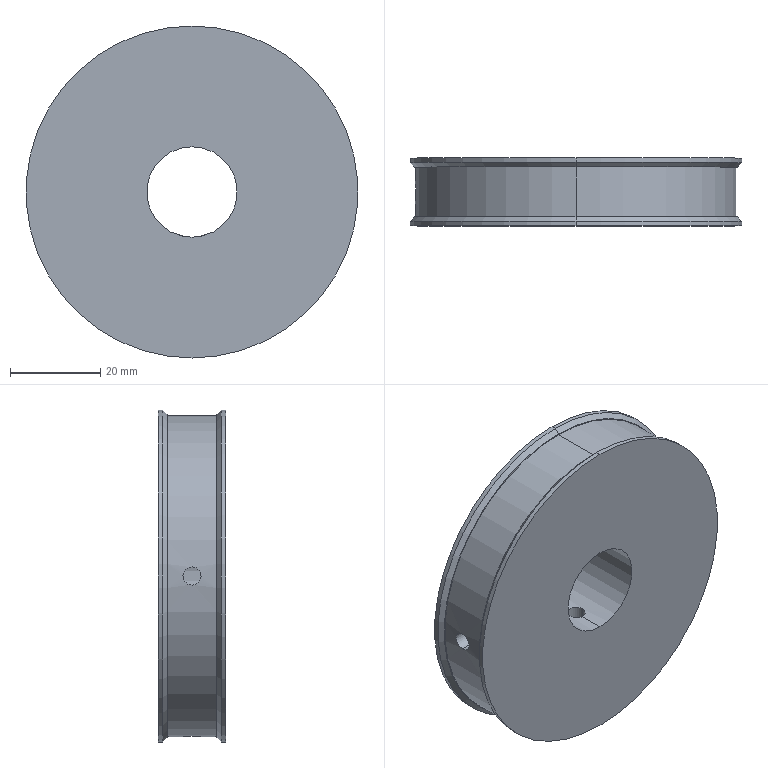Part | SolidWorks | features ICE 4, Chamfer 1, Extrusion 1 | 1 solid | 20 faces | box 73.4 x 15 x 73.4 mm | volume 54894 mm3 | cylinder 12 | cone 4 | plane 4 | commonest cylinder face diameters 4 x4 73.4 x4 20 x2 71 x2
STEP:
#1=CARTESIAN_POINT('',(-35.444,5.5,2.));
#2=VERTEX_POINT('',#1);
#3=CARTESIAN_POINT('',(-35.444,5.5,-2.));
#4=VERTEX_POINT('',#3);
#5=CARTESIAN_POINT('',(-35.444,5.5,2.));
#6=CARTESIAN_POINT('',(-35.444,5.239,2.));
#7=CARTESIAN_POINT('',(-35.447,4.976,1.948));
#8=CARTESIAN_POINT('',(-35.457,4.494,1.748));
#9=CARTESIAN_POINT('',(-35.464,4.271,1.599));
#10=CARTESIAN_POINT('',(-35.475,3.995,1.323));
#11=CARTESIAN_POINT('',(-35.479,3.91,1.22));
#12=CARTESIAN_POINT('',(-35.486,3.765,1.003));
#13=CARTESIAN_POINT('',(-35.489,3.703,0.8881));
#14=CARTESIAN_POINT('',(-35.494,3.603,0.6462));
#15=CARTESIAN_POINT('',(-35.496,3.564,0.5191));
#16=CARTESIAN_POINT('',(-35.499,3.513,0.2634));
#17=CARTESIAN_POINT('',(-35.5,3.5,0.1336));
#18=CARTESIAN_POINT('',(-35.5,3.5,-0.1303));
#19=CARTESIAN_POINT('',(-35.499,3.513,-0.2607));
#20=CARTESIAN_POINT('',(-35.496,3.563,-0.5163));
#21=CARTESIAN_POINT('',(-35.494,3.602,-0.6431));
#22=CARTESIAN_POINT('',(-35.489,3.702,-0.8856));
#23=CARTESIAN_POINT('',(-35.486,3.763,-1.001));
#24=CARTESIAN_POINT('',(-35.479,3.908,-1.218));
#25=CARTESIAN_POINT('',(-35.476,3.993,-1.321));
#26=CARTESIAN_POINT('',(-35.468,4.177,-1.506));
#27=CARTESIAN_POINT('',(-35.465,4.278,-1.588));
#28=CARTESIAN_POINT('',(-35.458,4.496,-1.735));
#29=CARTESIAN_POINT('',(-35.455,4.612,-1.797));
#30=CARTESIAN_POINT('',(-35.447,4.973,-1.947));
#31=CARTESIAN_POINT('',(-35.444,5.236,-2.));
#32=CARTESIAN_POINT('',(-35.444,5.5,-2.));
#33=B_SPLINE_CURVE_WITH_KNOTS('',3,(#5,#6,#7,#8,#9,#10,#11,#12,#13,#14,#15,#16,#17,#18,#19,#20,#21,#22,#23,#24,#25,#26,#27,#28,#29,#30,#31,#32),.UNSPECIFIED.,.F.,.F.,(4,2,2,2,2,2,2,2,2,2,2,2,2,4),(0.006254,0.007036,0.007817,0.008208,0.008599,0.00899,0.009381,0.009771,0.01016,0.01055,0.01094,0.01133,0.01173,0.01251),.UNSPECIFIED.);
#34=EDGE_CURVE('',#2,#4,#33,.T.);
#35=ORIENTED_EDGE('',*,*,#34,.F.);
#36=CARTESIAN_POINT('',(-9.798,5.5,2.));
#37=VERTEX_POINT('',#36);
#38=CARTESIAN_POINT('',(-43.,5.5,2.));
#39=DIRECTION('',(1.,0.,0.));
#40=VECTOR('',#39,1000.);
#41=LINE('',#38,#40);
#42=EDGE_CURVE('',#2,#37,#41,.T.);
#43=ORIENTED_EDGE('',*,*,#42,.T.);
#44=CARTESIAN_POINT('',(-9.798,5.5,-2.));
#45=VERTEX_POINT('',#44);
#46=CARTESIAN_POINT('',(-9.798,5.5,2.));
#47=CARTESIAN_POINT('',(-9.798,5.239,2.));
#48=CARTESIAN_POINT('',(-9.809,4.975,1.947));
#49=CARTESIAN_POINT('',(-9.837,4.614,1.798));
#50=CARTESIAN_POINT('',(-9.849,4.497,1.735));
#51=CARTESIAN_POINT('',(-9.873,4.279,1.59));
#52=CARTESIAN_POINT('',(-9.886,4.179,1.507));
#53=CARTESIAN_POINT('',(-9.913,3.994,1.323));
#54=CARTESIAN_POINT('',(-9.926,3.91,1.22));
#55=CARTESIAN_POINT('',(-9.95,3.765,1.004));
#56=CARTESIAN_POINT('',(-9.961,3.704,0.8892));
#57=CARTESIAN_POINT('',(-9.989,3.552,0.5252));
#58=CARTESIAN_POINT('',(-10.,3.5,0.2651));
#59=CARTESIAN_POINT('',(-10.,3.5,-0.131));
#60=CARTESIAN_POINT('',(-9.997,3.513,-0.2611));
#61=CARTESIAN_POINT('',(-9.987,3.564,-0.5174));
#62=CARTESIAN_POINT('',(-9.98,3.602,-0.645));
#63=CARTESIAN_POINT('',(-9.961,3.702,-0.8866));
#64=CARTESIAN_POINT('',(-9.95,3.764,-1.001));
#65=CARTESIAN_POINT('',(-9.926,3.909,-1.219));
#66=CARTESIAN_POINT('',(-9.913,3.993,-1.321));
#67=CARTESIAN_POINT('',(-9.873,4.269,-1.597));
#68=CARTESIAN_POINT('',(-9.847,4.491,-1.746));
#69=CARTESIAN_POINT('',(-9.819,4.852,-1.897));
#70=CARTESIAN_POINT('',(-9.811,4.979,-1.935));
#71=CARTESIAN_POINT('',(-9.801,5.237,-1.987));
#72=CARTESIAN_POINT('',(-9.798,5.368,-2.));
#73=CARTESIAN_POINT('',(-9.798,5.5,-2.));
#74=B_SPLINE_CURVE_WITH_KNOTS('',3,(#46,#47,#48,#49,#50,#51,#52,#53,#54,#55,#56,#57,#58,#59,#60,#61,#62,#63,#64,#65,#66,#67,#68,#69,#70,#71,#72,#73),.UNSPECIFIED.,.F.,.F.,(4,2,2,2,2,2,2,2,2,2,2,2,2,4),(0.006269,0.007052,0.007444,0.007835,0.008227,0.008619,0.009402,0.009794,0.01019,0.01058,0.01097,0.01175,0.01214,0.01254),.UNSPECIFIED.);
#75=EDGE_CURVE('',#37,#45,#74,.T.);
#76=ORIENTED_EDGE('',*,*,#75,.T.);
#77=CARTESIAN_POINT('',(-43.,5.5,-2.));
#78=DIRECTION('',(1.,0.,0.));
#79=VECTOR('',#78,1000.);
#80=LINE('',#77,#79);
#81=EDGE_CURVE('',#4,#45,#80,.T.);
#82=ORIENTED_EDGE('',*,*,#81,.F.);
#83=EDGE_LOOP('',(#35,#43,#76,#82));
#84=FACE_OUTER_BOUND('',#83,.T.);
#85=CARTESIAN_POINT('',(-43.,5.5,0.));
#86=DIRECTION('',(1.,0.,0.));
#87=DIRECTION('',(0.,0.,-1.));
#88=AXIS2_PLACEMENT_3D('',#85,#86,#87);
#89=CYLINDRICAL_SURFACE('',#88,2.);
#90=ADVANCED_FACE('',(#84),#89,.F.);
#91=CARTESIAN_POINT('',(-2.,5.5,-35.444));
#92=VERTEX_POINT('',#91);
#93=CARTESIAN_POINT('',(0.,3.5,-35.5));
#94=VERTEX_POINT('',#93);
#95=CARTESIAN_POINT('',(-2.,5.5,-35.444));
#96=CARTESIAN_POINT('',(-2.,5.37,-35.444));
#97=CARTESIAN_POINT('',(-1.987,5.237,-35.444));
#98=CARTESIAN_POINT('',(-1.936,4.981,-35.447));
#99=CARTESIAN_POINT('',(-1.898,4.856,-35.449));
#100=CARTESIAN_POINT('',(-1.798,4.614,-35.454));
#101=CARTESIAN_POINT('',(-1.735,4.497,-35.458));
#102=CARTESIAN_POINT('',(-1.59,4.28,-35.464));
#103=CARTESIAN_POINT('',(-1.508,4.179,-35.468));
#104=CARTESIAN_POINT('',(-1.321,3.992,-35.476));
#105=CARTESIAN_POINT('',(-1.22,3.91,-35.479));
#106=CARTESIAN_POINT('',(-1.003,3.765,-35.486));
#107=CARTESIAN_POINT('',(-0.8863,3.702,-35.489));
#108=CARTESIAN_POINT('',(-0.644,3.602,-35.494));
#109=CARTESIAN_POINT('',(-0.5193,3.564,-35.496));
#110=CARTESIAN_POINT('',(-0.2631,3.513,-35.499));
#111=CARTESIAN_POINT('',(-0.1305,3.5,-35.5));
#112=CARTESIAN_POINT('',(0.,3.5,-35.5));
#113=B_SPLINE_CURVE_WITH_KNOTS('',3,(#95,#96,#97,#98,#99,#100,#101,#102,#103,#104,#105,#106,#107,#108,#109,#110,#111,#112),.UNSPECIFIED.,.F.,.F.,(4,2,2,2,2,2,2,2,4),(0.003128,0.003519,0.003909,0.0043,0.004691,0.005082,0.005473,0.005863,0.006254),.UNSPECIFIED.);
#114=EDGE_CURVE('',#92,#94,#113,.T.);
#115=ORIENTED_EDGE('',*,*,#114,.F.);
#116=CARTESIAN_POINT('',(-2.,5.5,-9.798));
#117=VERTEX_POINT('',#116);
#118=CARTESIAN_POINT('',(-2.,5.5,-43.));
#119=DIRECTION('',(0.,0.,1.));
#120=VECTOR('',#119,1000.);
#121=LINE('',#118,#120);
#122=EDGE_CURVE('',#92,#117,#121,.T.);
#123=ORIENTED_EDGE('',*,*,#122,.T.);
#124=CARTESIAN_POINT('',(0.,3.5,-10.));
#125=VERTEX_POINT('',#124);
#126=CARTESIAN_POINT('',(-2.,5.5,-9.798));
#127=CARTESIAN_POINT('',(-2.,5.369,-9.798));
#128=CARTESIAN_POINT('',(-1.987,5.236,-9.801));
#129=CARTESIAN_POINT('',(-1.936,4.98,-9.811));
#130=CARTESIAN_POINT('',(-1.898,4.855,-9.818));
#131=CARTESIAN_POINT('',(-1.747,4.491,-9.847));
#132=CARTESIAN_POINT('',(-1.6,4.271,-9.873));
#133=CARTESIAN_POINT('',(-1.321,3.992,-9.913));
#134=CARTESIAN_POINT('',(-1.22,3.91,-9.926));
#135=CARTESIAN_POINT('',(-1.004,3.765,-9.95));
#136=CARTESIAN_POINT('',(-0.8868,3.703,-9.961));
#137=CARTESIAN_POINT('',(-0.6451,3.602,-9.98));
#138=CARTESIAN_POINT('',(-0.5204,3.564,-9.987));
#139=CARTESIAN_POINT('',(-0.2634,3.513,-9.997));
#140=CARTESIAN_POINT('',(-0.1307,3.5,-10.));
#141=CARTESIAN_POINT('',(0.,3.5,-10.));
#142=B_SPLINE_CURVE_WITH_KNOTS('',3,(#126,#127,#128,#129,#130,#131,#132,#133,#134,#135,#136,#137,#138,#139,#140,#141),.UNSPECIFIED.,.F.,.F.,(4,2,2,2,2,2,2,4),(0.003135,0.003527,0.003919,0.004702,0.005094,0.005485,0.005877,0.006269),.UNSPECIFIED.);
#143=EDGE_CURVE('',#117,#125,#142,.T.);
#144=ORIENTED_EDGE('',*,*,#143,.T.);
#145=CARTESIAN_POINT('',(2.,5.5,-9.798));
#146=VERTEX_POINT('',#145);
#147=CARTESIAN_POINT('',(0.,3.5,-10.));
#148=CARTESIAN_POINT('',(0.2614,3.5,-10.));
#149=CARTESIAN_POINT('',(0.5253,3.553,-9.989));
#150=CARTESIAN_POINT('',(0.8865,3.702,-9.961));
#151=CARTESIAN_POINT('',(1.003,3.765,-9.95));
#152=CARTESIAN_POINT('',(1.221,3.911,-9.926));
#153=CARTESIAN_POINT('',(1.322,3.993,-9.913));
#154=CARTESIAN_POINT('',(1.506,4.178,-9.886));
#155=CARTESIAN_POINT('',(1.59,4.28,-9.873));
#156=CARTESIAN_POINT('',(1.735,4.497,-9.849));
#157=CARTESIAN_POINT('',(1.797,4.611,-9.837));
#158=CARTESIAN_POINT('',(1.948,4.976,-9.809));
#159=CARTESIAN_POINT('',(2.,5.236,-9.798));
#160=CARTESIAN_POINT('',(2.,5.5,-9.798));
#161=B_SPLINE_CURVE_WITH_KNOTS('',3,(#147,#148,#149,#150,#151,#152,#153,#154,#155,#156,#157,#158,#159,#160),.UNSPECIFIED.,.F.,.F.,(4,2,2,2,2,2,4),(0.006269,0.007052,0.007444,0.007836,0.008228,0.00862,0.009403),.UNSPECIFIED.);
#162=EDGE_CURVE('',#125,#146,#161,.T.);
#163=ORIENTED_EDGE('',*,*,#162,.T.);
#164=CARTESIAN_POINT('',(2.,5.5,-35.444));
#165=VERTEX_POINT('',#164);
#166=CARTESIAN_POINT('',(2.,5.5,-43.));
#167=DIRECTION('',(0.,0.,1.));
#168=VECTOR('',#167,1000.);
#169=LINE('',#166,#168);
#170=EDGE_CURVE('',#165,#146,#169,.T.);
#171=ORIENTED_EDGE('',*,*,#170,.F.);
#172=CARTESIAN_POINT('',(0.,3.5,-35.5));
#173=CARTESIAN_POINT('',(0.2612,3.5,-35.5));
#174=CARTESIAN_POINT('',(0.5244,3.552,-35.497));
#175=CARTESIAN_POINT('',(1.006,3.752,-35.487));
#176=CARTESIAN_POINT('',(1.229,3.901,-35.479));
#177=CARTESIAN_POINT('',(1.506,4.178,-35.468));
#178=CARTESIAN_POINT('',(1.591,4.28,-35.464));
#179=CARTESIAN_POINT('',(1.736,4.498,-35.458));
#180=CARTESIAN_POINT('',(1.797,4.613,-35.455));
#181=CARTESIAN_POINT('',(1.898,4.855,-35.449));
#182=CARTESIAN_POINT('',(1.936,4.982,-35.447));
#183=CARTESIAN_POINT('',(1.987,5.238,-35.444));
#184=CARTESIAN_POINT('',(2.,5.368,-35.444));
#185=CARTESIAN_POINT('',(2.,5.5,-35.444));
#186=B_SPLINE_CURVE_WITH_KNOTS('',3,(#172,#173,#174,#175,#176,#177,#178,#179,#180,#181,#182,#183,#184,#185),.UNSPECIFIED.,.F.,.F.,(4,2,2,2,2,2,4),(0.006254,0.007036,0.007818,0.008209,0.0086,0.008991,0.009382),.UNSPECIFIED.);
#187=EDGE_CURVE('',#94,#165,#186,.T.);
#188=ORIENTED_EDGE('',*,*,#187,.F.);
#189=EDGE_LOOP('',(#115,#123,#144,#163,#171,#188));
#190=FACE_OUTER_BOUND('',#189,.T.);
#191=CARTESIAN_POINT('',(0.,5.5,-43.));
#192=DIRECTION('',(0.,0.,1.));
#193=DIRECTION('',(1.,0.,0.));
#194=AXIS2_PLACEMENT_3D('',#191,#192,#193);
#195=CYLINDRICAL_SURFACE('',#194,2.);
#196=ADVANCED_FACE('',(#190),#195,.F.);
#197=CARTESIAN_POINT('',(0.,11.,-35.7));
#198=VERTEX_POINT('',#197);
#199=CARTESIAN_POINT('',(0.,11.,35.7));
#200=VERTEX_POINT('',#199);
#201=CARTESIAN_POINT('',(0.,11.,0.));
#202=DIRECTION('',(0.,-1.,0.));
#203=DIRECTION('',(0.,0.,1.));
#204=AXIS2_PLACEMENT_3D('',#201,#202,#203);
#205=CIRCLE('',#204,35.7);
#206=EDGE_CURVE('',#198,#200,#205,.T.);
#207=ORIENTED_EDGE('',*,*,#206,.F.);
#208=CARTESIAN_POINT('',(0.,12.,-36.7));
#209=VERTEX_POINT('',#208);
#210=CARTESIAN_POINT('',(0.,12.,-36.7));
#211=DIRECTION('',(0.,0.7071,-0.7071));
#212=VECTOR('',#211,1000.);
#213=LINE('',#210,#212);
#214=EDGE_CURVE('',#198,#209,#213,.T.);
#215=ORIENTED_EDGE('',*,*,#214,.T.);
#216=CARTESIAN_POINT('',(0.,12.,36.7));
#217=VERTEX_POINT('',#216);
#218=CARTESIAN_POINT('',(0.,12.,0.));
#219=DIRECTION('',(0.,1.,0.));
#220=DIRECTION('',(0.,0.,1.));
#221=AXIS2_PLACEMENT_3D('',#218,#219,#220);
#222=CIRCLE('',#221,36.7);
#223=EDGE_CURVE('',#217,#209,#222,.T.);
#224=ORIENTED_EDGE('',*,*,#223,.F.);
#225=CARTESIAN_POINT('',(0.,12.,36.7));
#226=DIRECTION('',(0.,0.7071,0.7071));
#227=VECTOR('',#226,1000.);
#228=LINE('',#225,#227);
#229=EDGE_CURVE('',#200,#217,#228,.T.);
#230=ORIENTED_EDGE('',*,*,#229,.F.);
#231=EDGE_LOOP('',(#207,#215,#224,#230));
#232=FACE_OUTER_BOUND('',#231,.T.);
#233=CARTESIAN_POINT('',(0.,12.,0.));
#234=DIRECTION('',(0.,1.,0.));
#235=DIRECTION('',(0.,0.,1.));
#236=AXIS2_PLACEMENT_3D('',#233,#234,#235);
#237=CONICAL_SURFACE('',#236,36.7,0.7854);
#238=ADVANCED_FACE('',(#232),#237,.T.);
#239=CARTESIAN_POINT('',(0.,0.,35.7));
#240=VERTEX_POINT('',#239);
#241=CARTESIAN_POINT('',(0.,0.,-35.7));
#242=VERTEX_POINT('',#241);
#243=CARTESIAN_POINT('',(0.,0.,0.));
#244=DIRECTION('',(0.,1.,0.));
#245=DIRECTION('',(0.,0.,-1.));
#246=AXIS2_PLACEMENT_3D('',#243,#244,#245);
#247=CIRCLE('',#246,35.7);
#248=EDGE_CURVE('',#240,#242,#247,.T.);
#249=ORIENTED_EDGE('',*,*,#248,.F.);
#250=CARTESIAN_POINT('',(0.,-1.,36.7));
#251=VERTEX_POINT('',#250);
#252=CARTESIAN_POINT('',(0.,-1.,36.7));
#253=DIRECTION('',(0.,-0.7071,0.7071));
#254=VECTOR('',#253,1000.);
#255=LINE('',#252,#254);
#256=EDGE_CURVE('',#240,#251,#255,.T.);
#257=ORIENTED_EDGE('',*,*,#256,.T.);
#258=CARTESIAN_POINT('',(0.,-1.,-36.7));
#259=VERTEX_POINT('',#258);
#260=CARTESIAN_POINT('',(0.,-1.,0.));
#261=DIRECTION('',(0.,-1.,0.));
#262=DIRECTION('',(0.,0.,-1.));
#263=AXIS2_PLACEMENT_3D('',#260,#261,#262);
#264=CIRCLE('',#263,36.7);
#265=EDGE_CURVE('',#259,#251,#264,.T.);
#266=ORIENTED_EDGE('',*,*,#265,.F.);
#267=CARTESIAN_POINT('',(0.,-1.,-36.7));
#268=DIRECTION('',(0.,-0.7071,-0.7071));
#269=VECTOR('',#268,1000.);
#270=LINE('',#267,#269);
#271=EDGE_CURVE('',#242,#259,#270,.T.);
#272=ORIENTED_EDGE('',*,*,#271,.F.);
#273=EDGE_LOOP('',(#249,#257,#266,#272));
#274=FACE_OUTER_BOUND('',#273,.T.);
#275=CARTESIAN_POINT('',(0.,-1.,0.));
#276=DIRECTION('',(0.,-1.,0.));
#277=DIRECTION('',(0.,0.,-1.));
#278=AXIS2_PLACEMENT_3D('',#275,#276,#277);
#279=CONICAL_SURFACE('',#278,36.7,0.7854);
#280=ADVANCED_FACE('',(#274),#279,.T.);
#281=CARTESIAN_POINT('',(0.,-2.,-36.7));
#282=VERTEX_POINT('',#281);
#283=CARTESIAN_POINT('',(0.,-2.,36.7));
#284=VERTEX_POINT('',#283);
#285=CARTESIAN_POINT('',(0.,-2.,0.));
#286=DIRECTION('',(0.,-1.,0.));
#287=DIRECTION('',(0.,0.,-1.));
#288=AXIS2_PLACEMENT_3D('',#285,#286,#287);
#289=CIRCLE('',#288,36.7);
#290=EDGE_CURVE('',#282,#284,#289,.T.);
#291=ORIENTED_EDGE('',*,*,#290,.F.);
#292=CARTESIAN_POINT('',(0.,-2.,-36.7));
#293=DIRECTION('',(0.,1.,0.));
#294=VECTOR('',#293,1000.);
#295=LINE('',#292,#294);
#296=EDGE_CURVE('',#282,#259,#295,.T.);
#297=ORIENTED_EDGE('',*,*,#296,.T.);
#298=ORIENTED_EDGE('',*,*,#265,.T.);
#299=CARTESIAN_POINT('',(0.,-2.,36.7));
#300=DIRECTION('',(0.,1.,0.));
#301=VECTOR('',#300,1000.);
#302=LINE('',#299,#301);
#303=EDGE_CURVE('',#284,#251,#302,.T.);
#304=ORIENTED_EDGE('',*,*,#303,.F.);
#305=EDGE_LOOP('',(#291,#297,#298,#304));
#306=FACE_OUTER_BOUND('',#305,.T.);
#307=CARTESIAN_POINT('',(0.,-2.,0.));
#308=DIRECTION('',(0.,1.,0.));
#309=DIRECTION('',(0.,0.,1.));
#310=AXIS2_PLACEMENT_3D('',#307,#308,#309);
#311=CYLINDRICAL_SURFACE('',#310,36.7);
#312=ADVANCED_FACE('',(#306),#311,.T.);
#313=CARTESIAN_POINT('',(0.,13.,36.7));
#314=VERTEX_POINT('',#313);
#315=CARTESIAN_POINT('',(0.,13.,-36.7));
#316=VERTEX_POINT('',#315);
#317=CARTESIAN_POINT('',(0.,13.,0.));
#318=DIRECTION('',(0.,1.,0.));
#319=DIRECTION('',(0.,0.,1.));
#320=AXIS2_PLACEMENT_3D('',#317,#318,#319);
#321=CIRCLE('',#320,36.7);
#322=EDGE_CURVE('',#314,#316,#321,.T.);
#323=ORIENTED_EDGE('',*,*,#322,.F.);
#324=CARTESIAN_POINT('',(0.,13.,36.7));
#325=DIRECTION('',(0.,-1.,0.));
#326=VECTOR('',#325,1000.);
#327=LINE('',#324,#326);
#328=EDGE_CURVE('',#314,#217,#327,.T.);
#329=ORIENTED_EDGE('',*,*,#328,.T.);
#330=ORIENTED_EDGE('',*,*,#223,.T.);
#331=CARTESIAN_POINT('',(0.,13.,-36.7));
#332=DIRECTION('',(0.,-1.,0.));
#333=VECTOR('',#332,1000.);
#334=LINE('',#331,#333);
#335=EDGE_CURVE('',#316,#209,#334,.T.);
#336=ORIENTED_EDGE('',*,*,#335,.F.);
#337=EDGE_LOOP('',(#323,#329,#330,#336));
#338=FACE_OUTER_BOUND('',#337,.T.);
#339=CARTESIAN_POINT('',(0.,13.,0.));
#340=DIRECTION('',(0.,-1.,0.));
#341=DIRECTION('',(0.,0.,-1.));
#342=AXIS2_PLACEMENT_3D('',#339,#340,#341);
#343=CYLINDRICAL_SURFACE('',#342,36.7);
#344=ADVANCED_FACE('',(#338),#343,.T.);
#345=CARTESIAN_POINT('',(-9.798,5.5,-2.));
#346=CARTESIAN_POINT('',(-9.798,5.633,-2.));
#347=CARTESIAN_POINT('',(-9.801,5.763,-1.987));
#348=CARTESIAN_POINT('',(-9.811,6.019,-1.936));
#349=CARTESIAN_POINT('',(-9.818,6.146,-1.897));
#350=CARTESIAN_POINT('',(-9.837,6.388,-1.797));
#351=CARTESIAN_POINT('',(-9.849,6.503,-1.735));
#352=CARTESIAN_POINT('',(-9.873,6.72,-1.59));
#353=CARTESIAN_POINT('',(-9.886,6.823,-1.506));
#354=CARTESIAN_POINT('',(-9.926,7.098,-1.23));
#355=CARTESIAN_POINT('',(-9.952,7.247,-1.007));
#356=CARTESIAN_POINT('',(-9.989,7.447,-0.5261));
#357=CARTESIAN_POINT('',(-10.,7.5,-0.2624));
#358=CARTESIAN_POINT('',(-10.,7.5,0.13));
#359=CARTESIAN_POINT('',(-9.997,7.487,0.263));
#360=CARTESIAN_POINT('',(-9.987,7.436,0.5197));
#361=CARTESIAN_POINT('',(-9.98,7.398,0.6446));
#362=CARTESIAN_POINT('',(-9.952,7.247,1.008));
#363=CARTESIAN_POINT('',(-9.926,7.1,1.228));
#364=CARTESIAN_POINT('',(-9.886,6.821,1.507));
#365=CARTESIAN_POINT('',(-9.873,6.72,1.59));
#366=CARTESIAN_POINT('',(-9.849,6.504,1.735));
#367=CARTESIAN_POINT('',(-9.837,6.387,1.797));
#368=CARTESIAN_POINT('',(-9.818,6.145,1.898));
#369=CARTESIAN_POINT('',(-9.811,6.021,1.936));
#370=CARTESIAN_POINT('',(-9.801,5.763,1.987));
#371=CARTESIAN_POINT('',(-9.798,5.631,2.));
#372=CARTESIAN_POINT('',(-9.798,5.5,2.));
#373=B_SPLINE_CURVE_WITH_KNOTS('',3,(#345,#346,#347,#348,#349,#350,#351,#352,#353,#354,#355,#356,#357,#358,#359,#360,#361,#362,#363,#364,#365,#366,#367,#368,#369,#370,#371,#372),.UNSPECIFIED.,.F.,.F.,(4,2,2,2,2,2,2,2,2,2,2,2,2,4),(0.,0.0003918,0.0007836,0.001175,0.001567,0.002351,0.003134,0.003526,0.003918,0.004702,0.005093,0.005485,0.005877,0.006269),.UNSPECIFIED.);
#374=EDGE_CURVE('',#45,#37,#373,.T.);
#375=ORIENTED_EDGE('',*,*,#374,.F.);
#376=ORIENTED_EDGE('',*,*,#75,.F.);
#377=EDGE_LOOP('',(#375,#376));
#378=FACE_BOUND('',#377,.T.);
#379=CARTESIAN_POINT('',(0.,13.,-10.));
#380=VERTEX_POINT('',#379);
#381=CARTESIAN_POINT('',(0.,13.,10.));
#382=VERTEX_POINT('',#381);
#383=CARTESIAN_POINT('',(0.,13.,0.));
#384=DIRECTION('',(0.,1.,0.));
#385=DIRECTION('',(0.,0.,1.));
#386=AXIS2_PLACEMENT_3D('',#383,#384,#385);
#387=CIRCLE('',#386,10.);
#388=EDGE_CURVE('',#380,#382,#387,.T.);
#389=ORIENTED_EDGE('',*,*,#388,.T.);
#390=CARTESIAN_POINT('',(0.,-2.,10.));
#391=VERTEX_POINT('',#390);
#392=CARTESIAN_POINT('',(0.,11.,10.));
#393=DIRECTION('',(0.,-1.,0.));
#394=VECTOR('',#393,1000.);
#395=LINE('',#392,#394);
#396=EDGE_CURVE('',#382,#391,#395,.T.);
#397=ORIENTED_EDGE('',*,*,#396,.T.);
#398=CARTESIAN_POINT('',(0.,-2.,-10.));
#399=VERTEX_POINT('',#398);
#400=CARTESIAN_POINT('',(0.,-2.,0.));
#401=DIRECTION('',(0.,-1.,0.));
#402=DIRECTION('',(0.,0.,-1.));
#403=AXIS2_PLACEMENT_3D('',#400,#401,#402);
#404=CIRCLE('',#403,10.);
#405=EDGE_CURVE('',#391,#399,#404,.T.);
#406=ORIENTED_EDGE('',*,*,#405,.T.);
#407=CARTESIAN_POINT('',(0.,11.,-10.));
#408=DIRECTION('',(0.,-1.,0.));
#409=VECTOR('',#408,1000.);
#410=LINE('',#407,#409);
#411=EDGE_CURVE('',#125,#399,#410,.T.);
#412=ORIENTED_EDGE('',*,*,#411,.F.);
#413=ORIENTED_EDGE('',*,*,#143,.F.);
#414=CARTESIAN_POINT('',(0.,7.5,-10.));
#415=VERTEX_POINT('',#414);
#416=CARTESIAN_POINT('',(0.,7.5,-10.));
#417=CARTESIAN_POINT('',(-0.1325,7.5,-10.));
#418=CARTESIAN_POINT('',(-0.2628,7.487,-9.997));
#419=CARTESIAN_POINT('',(-0.5189,7.436,-9.987));
#420=CARTESIAN_POINT('',(-0.6462,7.397,-9.98));
#421=CARTESIAN_POINT('',(-0.8883,7.297,-9.961));
#422=CARTESIAN_POINT('',(-1.003,7.235,-9.95));
#423=CARTESIAN_POINT('',(-1.22,7.09,-9.926));
#424=CARTESIAN_POINT('',(-1.323,7.006,-9.913));
#425=CARTESIAN_POINT('',(-1.599,6.729,-9.873));
#426=CARTESIAN_POINT('',(-1.748,6.507,-9.847));
#427=CARTESIAN_POINT('',(-1.947,6.025,-9.809));
#428=CARTESIAN_POINT('',(-2.,5.762,-9.798));
#429=CARTESIAN_POINT('',(-2.,5.5,-9.798));
#430=B_SPLINE_CURVE_WITH_KNOTS('',3,(#416,#417,#418,#419,#420,#421,#422,#423,#424,#425,#426,#427,#428,#429),.UNSPECIFIED.,.F.,.F.,(4,2,2,2,2,2,4),(0.,0.0003919,0.0007838,0.001176,0.001568,0.002351,0.003135),.UNSPECIFIED.);
#431=EDGE_CURVE('',#415,#117,#430,.T.);
#432=ORIENTED_EDGE('',*,*,#431,.F.);
#433=CARTESIAN_POINT('',(0.,11.,-10.));
#434=DIRECTION('',(0.,-1.,0.));
#435=VECTOR('',#434,1000.);
#436=LINE('',#433,#435);
#437=EDGE_CURVE('',#380,#415,#436,.T.);
#438=ORIENTED_EDGE('',*,*,#437,.F.);
#439=EDGE_LOOP('',(#389,#397,#406,#412,#413,#432,#438));
#440=FACE_OUTER_BOUND('',#439,.T.);
#441=CARTESIAN_POINT('',(0.,11.,0.));
#442=DIRECTION('',(0.,-1.,0.));
#443=DIRECTION('',(0.,0.,-1.));
#444=AXIS2_PLACEMENT_3D('',#441,#442,#443);
#445=CYLINDRICAL_SURFACE('',#444,10.);
#446=ADVANCED_FACE('',(#378,#440),#445,.F.);
#447=CARTESIAN_POINT('',(0.,11.,35.5));
#448=VERTEX_POINT('',#447);
#449=CARTESIAN_POINT('',(0.,11.,-35.5));
#450=VERTEX_POINT('',#449);
#451=CARTESIAN_POINT('',(0.,11.,0.));
#452=DIRECTION('',(0.,1.,0.));
#453=DIRECTION('',(0.,0.,1.));
#454=AXIS2_PLACEMENT_3D('',#451,#452,#453);
#455=CIRCLE('',#454,35.5);
#456=EDGE_CURVE('',#448,#450,#455,.T.);
#457=ORIENTED_EDGE('',*,*,#456,.F.);
#458=CARTESIAN_POINT('',(0.,0.,35.5));
#459=VERTEX_POINT('',#458);
#460=CARTESIAN_POINT('',(0.,11.,35.5));
#461=DIRECTION('',(0.,-1.,0.));
#462=VECTOR('',#461,1000.);
#463=LINE('',#460,#462);
#464=EDGE_CURVE('',#448,#459,#463,.T.);
#465=ORIENTED_EDGE('',*,*,#464,.T.);
#466=CARTESIAN_POINT('',(0.,0.,-35.5));
#467=VERTEX_POINT('',#466);
#468=CARTESIAN_POINT('',(0.,0.,0.));
#469=DIRECTION('',(0.,-1.,0.));
#470=DIRECTION('',(0.,0.,-1.));
#471=AXIS2_PLACEMENT_3D('',#468,#469,#470);
#472=CIRCLE('',#471,35.5);
#473=EDGE_CURVE('',#467,#459,#472,.T.);
#474=ORIENTED_EDGE('',*,*,#473,.F.);
#475=CARTESIAN_POINT('',(0.,11.,-35.5));
#476=DIRECTION('',(0.,-1.,0.));
#477=VECTOR('',#476,1000.);
#478=LINE('',#475,#477);
#479=EDGE_CURVE('',#94,#467,#478,.T.);
#480=ORIENTED_EDGE('',*,*,#479,.F.);
#481=ORIENTED_EDGE('',*,*,#187,.T.);
#482=CARTESIAN_POINT('',(0.,7.5,-35.5));
#483=VERTEX_POINT('',#482);
#484=CARTESIAN_POINT('',(2.,5.5,-35.444));
#485=CARTESIAN_POINT('',(2.,5.632,-35.444));
#486=CARTESIAN_POINT('',(1.987,5.762,-35.444));
#487=CARTESIAN_POINT('',(1.936,6.018,-35.447));
#488=CARTESIAN_POINT('',(1.898,6.144,-35.449));
#489=CARTESIAN_POINT('',(1.798,6.387,-35.454));
#490=CARTESIAN_POINT('',(1.736,6.501,-35.458));
#491=CARTESIAN_POINT('',(1.591,6.719,-35.464));
#492=CARTESIAN_POINT('',(1.507,6.822,-35.468));
#493=CARTESIAN_POINT('',(1.322,7.006,-35.475));
#494=CARTESIAN_POINT('',(1.222,7.089,-35.479));
#495=CARTESIAN_POINT('',(1.004,7.235,-35.486));
#496=CARTESIAN_POINT('',(0.8872,7.297,-35.489));
#497=CARTESIAN_POINT('',(0.5266,7.447,-35.497));
#498=CARTESIAN_POINT('',(0.2641,7.5,-35.5));
#499=CARTESIAN_POINT('',(0.,7.5,-35.5));
#500=B_SPLINE_CURVE_WITH_KNOTS('',3,(#484,#485,#486,#487,#488,#489,#490,#491,#492,#493,#494,#495,#496,#497,#498,#499),.UNSPECIFIED.,.F.,.F.,(4,2,2,2,2,2,2,4),(0.009382,0.009773,0.01016,0.01055,0.01094,0.01134,0.01173,0.01251),.UNSPECIFIED.);
#501=EDGE_CURVE('',#165,#483,#500,.T.);
#502=ORIENTED_EDGE('',*,*,#501,.T.);
#503=CARTESIAN_POINT('',(0.,11.,-35.5));
#504=DIRECTION('',(0.,-1.,0.));
#505=VECTOR('',#504,1000.);
#506=LINE('',#503,#505);
#507=EDGE_CURVE('',#450,#483,#506,.T.);
#508=ORIENTED_EDGE('',*,*,#507,.F.);
#509=EDGE_LOOP('',(#457,#465,#474,#480,#481,#502,#508));
#510=FACE_OUTER_BOUND('',#509,.T.);
#511=CARTESIAN_POINT('',(0.,11.,0.));
#512=DIRECTION('',(0.,-1.,0.));
#513=DIRECTION('',(0.,0.,-1.));
#514=AXIS2_PLACEMENT_3D('',#511,#512,#513);
#515=CYLINDRICAL_SURFACE('',#514,35.5);
#516=ADVANCED_FACE('',(#510),#515,.T.);
#517=ORIENTED_EDGE('',*,*,#464,.F.);
#518=CARTESIAN_POINT('',(0.,11.,0.));
#519=DIRECTION('',(0.,1.,0.));
#520=DIRECTION('',(0.,0.,1.));
#521=AXIS2_PLACEMENT_3D('',#518,#519,#520);
#522=CIRCLE('',#521,35.5);
#523=EDGE_CURVE('',#450,#448,#522,.T.);
#524=ORIENTED_EDGE('',*,*,#523,.F.);
#525=ORIENTED_EDGE('',*,*,#507,.T.);
#526=CARTESIAN_POINT('',(0.,7.5,-35.5));
#527=CARTESIAN_POINT('',(-0.1322,7.5,-35.5));
#528=CARTESIAN_POINT('',(-0.2622,7.487,-35.499));
#529=CARTESIAN_POINT('',(-0.5179,7.436,-35.496));
#530=CARTESIAN_POINT('',(-0.645,7.398,-35.494));
#531=CARTESIAN_POINT('',(-0.8872,7.297,-35.489));
#532=CARTESIAN_POINT('',(-1.002,7.236,-35.486));
#533=CARTESIAN_POINT('',(-1.22,7.091,-35.479));
#534=CARTESIAN_POINT('',(-1.322,7.006,-35.475));
#535=CARTESIAN_POINT('',(-1.599,6.729,-35.464));
#536=CARTESIAN_POINT('',(-1.748,6.506,-35.457));
#537=CARTESIAN_POINT('',(-1.948,6.024,-35.447));
#538=CARTESIAN_POINT('',(-2.,5.761,-35.444));
#539=CARTESIAN_POINT('',(-2.,5.5,-35.444));
#540=B_SPLINE_CURVE_WITH_KNOTS('',3,(#526,#527,#528,#529,#530,#531,#532,#533,#534,#535,#536,#537,#538,#539),.UNSPECIFIED.,.F.,.F.,(4,2,2,2,2,2,4),(0.,0.000391,0.0007819,0.001173,0.001564,0.002346,0.003128),.UNSPECIFIED.);
#541=EDGE_CURVE('',#483,#92,#540,.T.);
#542=ORIENTED_EDGE('',*,*,#541,.T.);
#543=ORIENTED_EDGE('',*,*,#114,.T.);
#544=ORIENTED_EDGE('',*,*,#479,.T.);
#545=CARTESIAN_POINT('',(0.,0.,0.));
#546=DIRECTION('',(0.,-1.,0.));
#547=DIRECTION('',(0.,0.,-1.));
#548=AXIS2_PLACEMENT_3D('',#545,#546,#547);
#549=CIRCLE('',#548,35.5);
#550=EDGE_CURVE('',#459,#467,#549,.T.);
#551=ORIENTED_EDGE('',*,*,#550,.F.);
#552=EDGE_LOOP('',(#517,#524,#525,#542,#543,#544,#551));
#553=FACE_OUTER_BOUND('',#552,.T.);
#554=CARTESIAN_POINT('',(-35.444,5.5,-2.));
#555=CARTESIAN_POINT('',(-35.444,5.632,-2.));
#556=CARTESIAN_POINT('',(-35.444,5.762,-1.987));
#557=CARTESIAN_POINT('',(-35.447,6.018,-1.936));
#558=CARTESIAN_POINT('',(-35.449,6.145,-1.898));
#559=CARTESIAN_POINT('',(-35.455,6.387,-1.797));
#560=CARTESIAN_POINT('',(-35.458,6.502,-1.736));
#561=CARTESIAN_POINT('',(-35.464,6.719,-1.591));
#562=CARTESIAN_POINT('',(-35.468,6.822,-1.506));
#563=CARTESIAN_POINT('',(-35.479,7.099,-1.229));
#564=CARTESIAN_POINT('',(-35.487,7.248,-1.006));
#565=CARTESIAN_POINT('',(-35.497,7.447,-0.5249));
#566=CARTESIAN_POINT('',(-35.5,7.5,-0.2617));
#567=CARTESIAN_POINT('',(-35.5,7.5,0.1298));
#568=CARTESIAN_POINT('',(-35.499,7.487,0.2623));
#569=CARTESIAN_POINT('',(-35.496,7.436,0.5188));
#570=CARTESIAN_POINT('',(-35.494,7.398,0.6435));
#571=CARTESIAN_POINT('',(-35.489,7.298,0.8857));
#572=CARTESIAN_POINT('',(-35.486,7.235,1.003));
#573=CARTESIAN_POINT('',(-35.479,7.091,1.22));
#574=CARTESIAN_POINT('',(-35.476,7.008,1.321));
#575=CARTESIAN_POINT('',(-35.468,6.821,1.507));
#576=CARTESIAN_POINT('',(-35.464,6.72,1.59));
#577=CARTESIAN_POINT('',(-35.458,6.503,1.735));
#578=CARTESIAN_POINT('',(-35.454,6.387,1.798));
#579=CARTESIAN_POINT('',(-35.449,6.144,1.898));
#580=CARTESIAN_POINT('',(-35.447,6.019,1.936));
#581=CARTESIAN_POINT('',(-35.444,5.763,1.987));
#582=CARTESIAN_POINT('',(-35.444,5.631,2.));
#583=CARTESIAN_POINT('',(-35.444,5.5,2.));
#584=B_SPLINE_CURVE_WITH_KNOTS('',3,(#554,#555,#556,#557,#558,#559,#560,#561,#562,#563,#564,#565,#566,#567,#568,#569,#570,#571,#572,#573,#574,#575,#576,#577,#578,#579,#580,#581,#582,#583),.UNSPECIFIED.,.F.,.F.,(4,2,2,2,2,2,2,2,2,2,2,2,2,2,4),(0.,0.0003909,0.0007818,0.001173,0.001564,0.002345,0.003127,0.003518,0.003909,0.0043,0.004691,0.005081,0.005472,0.005863,0.006254),.UNSPECIFIED.);
#585=EDGE_CURVE('',#4,#2,#584,.T.);
#586=ORIENTED_EDGE('',*,*,#585,.T.);
#587=ORIENTED_EDGE('',*,*,#34,.T.);
#588=EDGE_LOOP('',(#586,#587));
#589=FACE_BOUND('',#588,.T.);
#590=CARTESIAN_POINT('',(0.,11.,0.));
#591=DIRECTION('',(0.,-1.,0.));
#592=DIRECTION('',(0.,0.,-1.));
#593=AXIS2_PLACEMENT_3D('',#590,#591,#592);
#594=CYLINDRICAL_SURFACE('',#593,35.5);
#595=ADVANCED_FACE('',(#553,#589),#594,.T.);
#596=ORIENTED_EDGE('',*,*,#396,.F.);
#597=CARTESIAN_POINT('',(0.,13.,0.));
#598=DIRECTION('',(0.,1.,0.));
#599=DIRECTION('',(0.,0.,1.));
#600=AXIS2_PLACEMENT_3D('',#597,#598,#599);
#601=CIRCLE('',#600,10.);
#602=EDGE_CURVE('',#382,#380,#601,.T.);
#603=ORIENTED_EDGE('',*,*,#602,.T.);
#604=ORIENTED_EDGE('',*,*,#437,.T.);
#605=CARTESIAN_POINT('',(2.,5.5,-9.798));
#606=CARTESIAN_POINT('',(2.,5.632,-9.798));
#607=CARTESIAN_POINT('',(1.987,5.762,-9.801));
#608=CARTESIAN_POINT('',(1.936,6.018,-9.811));
#609=CARTESIAN_POINT('',(1.897,6.146,-9.818));
#610=CARTESIAN_POINT('',(1.797,6.387,-9.837));
#611=CARTESIAN_POINT('',(1.736,6.502,-9.848));
#612=CARTESIAN_POINT('',(1.591,6.72,-9.873));
#613=CARTESIAN_POINT('',(1.507,6.822,-9.886));
#614=CARTESIAN_POINT('',(1.231,7.097,-9.926));
#615=CARTESIAN_POINT('',(1.009,7.247,-9.952));
#616=CARTESIAN_POINT('',(0.648,7.397,-9.98));
#617=CARTESIAN_POINT('',(0.5212,7.435,-9.987));
#618=CARTESIAN_POINT('',(0.2631,7.487,-9.997));
#619=CARTESIAN_POINT('',(0.1324,7.5,-10.));
#620=CARTESIAN_POINT('',(0.,7.5,-10.));
#621=B_SPLINE_CURVE_WITH_KNOTS('',3,(#605,#606,#607,#608,#609,#610,#611,#612,#613,#614,#615,#616,#617,#618,#619,#620),.UNSPECIFIED.,.F.,.F.,(4,2,2,2,2,2,2,4),(0.009403,0.009795,0.01019,0.01058,0.01097,0.01175,0.01214,0.01254),.UNSPECIFIED.);
#622=EDGE_CURVE('',#146,#415,#621,.T.);
#623=ORIENTED_EDGE('',*,*,#622,.F.);
#624=ORIENTED_EDGE('',*,*,#162,.F.);
#625=ORIENTED_EDGE('',*,*,#411,.T.);
#626=CARTESIAN_POINT('',(0.,-2.,0.));
#627=DIRECTION('',(0.,-1.,0.));
#628=DIRECTION('',(0.,0.,-1.));
#629=AXIS2_PLACEMENT_3D('',#626,#627,#628);
#630=CIRCLE('',#629,10.);
#631=EDGE_CURVE('',#399,#391,#630,.T.);
#632=ORIENTED_EDGE('',*,*,#631,.T.);
#633=EDGE_LOOP('',(#596,#603,#604,#623,#624,#625,#632));
#634=FACE_OUTER_BOUND('',#633,.T.);
#635=CARTESIAN_POINT('',(0.,11.,0.));
#636=DIRECTION('',(0.,-1.,0.));
#637=DIRECTION('',(0.,0.,-1.));
#638=AXIS2_PLACEMENT_3D('',#635,#636,#637);
#639=CYLINDRICAL_SURFACE('',#638,10.);
#640=ADVANCED_FACE('',(#634),#639,.F.);
#641=CARTESIAN_POINT('',(0.,11.,0.));
#642=DIRECTION('',(0.,-1.,0.));
#643=DIRECTION('',(0.,0.,1.));
#644=AXIS2_PLACEMENT_3D('',#641,#642,#643);
#645=CIRCLE('',#644,35.7);
#646=EDGE_CURVE('',#200,#198,#645,.T.);
#647=ORIENTED_EDGE('',*,*,#646,.T.);
#648=ORIENTED_EDGE('',*,*,#206,.T.);
#649=EDGE_LOOP('',(#647,#648));
#650=FACE_OUTER_BOUND('',#649,.T.);
#651=ORIENTED_EDGE('',*,*,#523,.T.);
#652=ORIENTED_EDGE('',*,*,#456,.T.);
#653=EDGE_LOOP('',(#651,#652));
#654=FACE_BOUND('',#653,.T.);
#655=CARTESIAN_POINT('',(0.,11.,0.));
#656=DIRECTION('',(0.,1.,0.));
#657=DIRECTION('',(0.,0.,1.));
#658=AXIS2_PLACEMENT_3D('',#655,#656,#657);
#659=PLANE('',#658);
#660=ADVANCED_FACE('',(#650,#654),#659,.F.);
#661=CARTESIAN_POINT('',(0.,13.,0.));
#662=DIRECTION('',(0.,1.,0.));
#663=DIRECTION('',(0.,0.,1.));
#664=AXIS2_PLACEMENT_3D('',#661,#662,#663);
#665=CIRCLE('',#664,36.7);
#666=EDGE_CURVE('',#316,#314,#665,.T.);
#667=ORIENTED_EDGE('',*,*,#666,.T.);
#668=ORIENTED_EDGE('',*,*,#322,.T.);
#669=EDGE_LOOP('',(#667,#668));
#670=FACE_OUTER_BOUND('',#669,.T.);
#671=ORIENTED_EDGE('',*,*,#388,.F.);
#672=ORIENTED_EDGE('',*,*,#602,.F.);
#673=EDGE_LOOP('',(#671,#672));
#674=FACE_BOUND('',#673,.T.);
#675=CARTESIAN_POINT('',(0.,13.,0.));
#676=DIRECTION('',(0.,1.,0.));
#677=DIRECTION('',(0.,0.,1.));
#678=AXIS2_PLACEMENT_3D('',#675,#676,#677);
#679=PLANE('',#678);
#680=ADVANCED_FACE('',(#670,#674),#679,.T.);
#681=ORIENTED_EDGE('',*,*,#328,.F.);
#682=ORIENTED_EDGE('',*,*,#666,.F.);
#683=ORIENTED_EDGE('',*,*,#335,.T.);
#684=CARTESIAN_POINT('',(0.,12.,0.));
#685=DIRECTION('',(0.,1.,0.));
#686=DIRECTION('',(0.,0.,1.));
#687=AXIS2_PLACEMENT_3D('',#684,#685,#686);
#688=CIRCLE('',#687,36.7);
#689=EDGE_CURVE('',#209,#217,#688,.T.);
#690=ORIENTED_EDGE('',*,*,#689,.T.);
#691=EDGE_LOOP('',(#681,#682,#683,#690));
#692=FACE_OUTER_BOUND('',#691,.T.);
#693=CARTESIAN_POINT('',(0.,13.,0.));
#694=DIRECTION('',(0.,-1.,0.));
#695=DIRECTION('',(0.,0.,-1.));
#696=AXIS2_PLACEMENT_3D('',#693,#694,#695);
#697=CYLINDRICAL_SURFACE('',#696,36.7);
#698=ADVANCED_FACE('',(#692),#697,.T.);
#699=CARTESIAN_POINT('',(0.,0.,0.));
#700=DIRECTION('',(0.,1.,0.));
#701=DIRECTION('',(0.,0.,-1.));
#702=AXIS2_PLACEMENT_3D('',#699,#700,#701);
#703=CIRCLE('',#702,35.7);
#704=EDGE_CURVE('',#242,#240,#703,.T.);
#705=ORIENTED_EDGE('',*,*,#704,.T.);
#706=ORIENTED_EDGE('',*,*,#248,.T.);
#707=EDGE_LOOP('',(#705,#706));
#708=FACE_OUTER_BOUND('',#707,.T.);
#709=ORIENTED_EDGE('',*,*,#473,.T.);
#710=ORIENTED_EDGE('',*,*,#550,.T.);
#711=EDGE_LOOP('',(#709,#710));
#712=FACE_BOUND('',#711,.T.);
#713=CARTESIAN_POINT('',(0.,0.,0.));
#714=DIRECTION('',(0.,-1.,0.));
#715=DIRECTION('',(0.,0.,-1.));
#716=AXIS2_PLACEMENT_3D('',#713,#714,#715);
#717=PLANE('',#716);
#718=ADVANCED_FACE('',(#708,#712),#717,.F.);
#719=CARTESIAN_POINT('',(0.,-2.,0.));
#720=DIRECTION('',(0.,-1.,0.));
#721=DIRECTION('',(0.,0.,-1.));
#722=AXIS2_PLACEMENT_3D('',#719,#720,#721);
#723=CIRCLE('',#722,36.7);
#724=EDGE_CURVE('',#284,#282,#723,.T.);
#725=ORIENTED_EDGE('',*,*,#724,.T.);
#726=ORIENTED_EDGE('',*,*,#290,.T.);
#727=EDGE_LOOP('',(#725,#726));
#728=FACE_OUTER_BOUND('',#727,.T.);
#729=ORIENTED_EDGE('',*,*,#631,.F.);
#730=ORIENTED_EDGE('',*,*,#405,.F.);
#731=EDGE_LOOP('',(#729,#730));
#732=FACE_BOUND('',#731,.T.);
#733=CARTESIAN_POINT('',(0.,-2.,0.));
#734=DIRECTION('',(0.,-1.,0.));
#735=DIRECTION('',(0.,0.,-1.));
#736=AXIS2_PLACEMENT_3D('',#733,#734,#735);
#737=PLANE('',#736);
#738=ADVANCED_FACE('',(#728,#732),#737,.T.);
#739=ORIENTED_EDGE('',*,*,#296,.F.);
#740=ORIENTED_EDGE('',*,*,#724,.F.);
#741=ORIENTED_EDGE('',*,*,#303,.T.);
#742=CARTESIAN_POINT('',(0.,-1.,0.));
#743=DIRECTION('',(0.,-1.,0.));
#744=DIRECTION('',(0.,0.,-1.));
#745=AXIS2_PLACEMENT_3D('',#742,#743,#744);
#746=CIRCLE('',#745,36.7);
#747=EDGE_CURVE('',#251,#259,#746,.T.);
#748=ORIENTED_EDGE('',*,*,#747,.T.);
#749=EDGE_LOOP('',(#739,#740,#741,#748));
#750=FACE_OUTER_BOUND('',#749,.T.);
#751=CARTESIAN_POINT('',(0.,-2.,0.));
#752=DIRECTION('',(0.,1.,0.));
#753=DIRECTION('',(0.,0.,1.));
#754=AXIS2_PLACEMENT_3D('',#751,#752,#753);
#755=CYLINDRICAL_SURFACE('',#754,36.7);
#756=ADVANCED_FACE('',(#750),#755,.T.);
#757=ORIENTED_EDGE('',*,*,#256,.F.);
#758=ORIENTED_EDGE('',*,*,#704,.F.);
#759=ORIENTED_EDGE('',*,*,#271,.T.);
#760=ORIENTED_EDGE('',*,*,#747,.F.);
#761=EDGE_LOOP('',(#757,#758,#759,#760));
#762=FACE_OUTER_BOUND('',#761,.T.);
#763=CARTESIAN_POINT('',(0.,-1.,0.));
#764=DIRECTION('',(0.,-1.,0.));
#765=DIRECTION('',(0.,0.,-1.));
#766=AXIS2_PLACEMENT_3D('',#763,#764,#765);
#767=CONICAL_SURFACE('',#766,36.7,0.7854);
#768=ADVANCED_FACE('',(#762),#767,.T.);
#769=ORIENTED_EDGE('',*,*,#214,.F.);
#770=ORIENTED_EDGE('',*,*,#646,.F.);
#771=ORIENTED_EDGE('',*,*,#229,.T.);
#772=ORIENTED_EDGE('',*,*,#689,.F.);
#773=EDGE_LOOP('',(#769,#770,#771,#772));
#774=FACE_OUTER_BOUND('',#773,.T.);
#775=CARTESIAN_POINT('',(0.,12.,0.));
#776=DIRECTION('',(0.,1.,0.));
#777=DIRECTION('',(0.,0.,1.));
#778=AXIS2_PLACEMENT_3D('',#775,#776,#777);
#779=CONICAL_SURFACE('',#778,36.7,0.7854);
#780=ADVANCED_FACE('',(#774),#779,.T.);
#781=ORIENTED_EDGE('',*,*,#122,.F.);
#782=ORIENTED_EDGE('',*,*,#541,.F.);
#783=ORIENTED_EDGE('',*,*,#501,.F.);
#784=ORIENTED_EDGE('',*,*,#170,.T.);
#785=ORIENTED_EDGE('',*,*,#622,.T.);
#786=ORIENTED_EDGE('',*,*,#431,.T.);
#787=EDGE_LOOP('',(#781,#782,#783,#784,#785,#786));
#788=FACE_OUTER_BOUND('',#787,.T.);
#789=CARTESIAN_POINT('',(0.,5.5,-43.));
#790=DIRECTION('',(0.,0.,1.));
#791=DIRECTION('',(1.,0.,0.));
#792=AXIS2_PLACEMENT_3D('',#789,#790,#791);
#793=CYLINDRICAL_SURFACE('',#792,2.);
#794=ADVANCED_FACE('',(#788),#793,.F.);
#795=ORIENTED_EDGE('',*,*,#42,.F.);
#796=ORIENTED_EDGE('',*,*,#585,.F.);
#797=ORIENTED_EDGE('',*,*,#81,.T.);
#798=ORIENTED_EDGE('',*,*,#374,.T.);
#799=EDGE_LOOP('',(#795,#796,#797,#798));
#800=FACE_OUTER_BOUND('',#799,.T.);
#801=CARTESIAN_POINT('',(-43.,5.5,0.));
#802=DIRECTION('',(1.,0.,0.));
#803=DIRECTION('',(0.,0.,-1.));
#804=AXIS2_PLACEMENT_3D('',#801,#802,#803);
#805=CYLINDRICAL_SURFACE('',#804,2.);
#806=ADVANCED_FACE('',(#800),#805,.F.);
#807=CLOSED_SHELL('',(#90,#196,#238,#280,#312,#344,#446,#516,#595,#640,#660,#680,#698,#718,#738,#756,#768,#780,#794,#806));
#808=MANIFOLD_SOLID_BREP('',#807);
#809=CARTESIAN_POINT('',(0.,0.,0.));
#810=DIRECTION('',(0.,0.,1.));
#811=DIRECTION('',(1.,0.,0.));
#812=AXIS2_PLACEMENT_3D('',#809,#810,#811);
#813=(LENGTH_UNIT()NAMED_UNIT(*)SI_UNIT(.MILLI.,.METRE.));
#814=UNCERTAINTY_MEASURE_WITH_UNIT(LENGTH_MEASURE(0.00001),#813,'','');
#815=(NAMED_UNIT(*)PLANE_ANGLE_UNIT()SI_UNIT($,.RADIAN.));
#816=(NAMED_UNIT(*)SI_UNIT($,.STERADIAN.)SOLID_ANGLE_UNIT());
#817=(GEOMETRIC_REPRESENTATION_CONTEXT(3)GLOBAL_UNCERTAINTY_ASSIGNED_CONTEXT((#814))GLOBAL_UNIT_ASSIGNED_CONTEXT((#813,#815,#816))REPRESENTATION_CONTEXT('',''));
#818=ADVANCED_BREP_SHAPE_REPRESENTATION('',(#808,#812),#817);